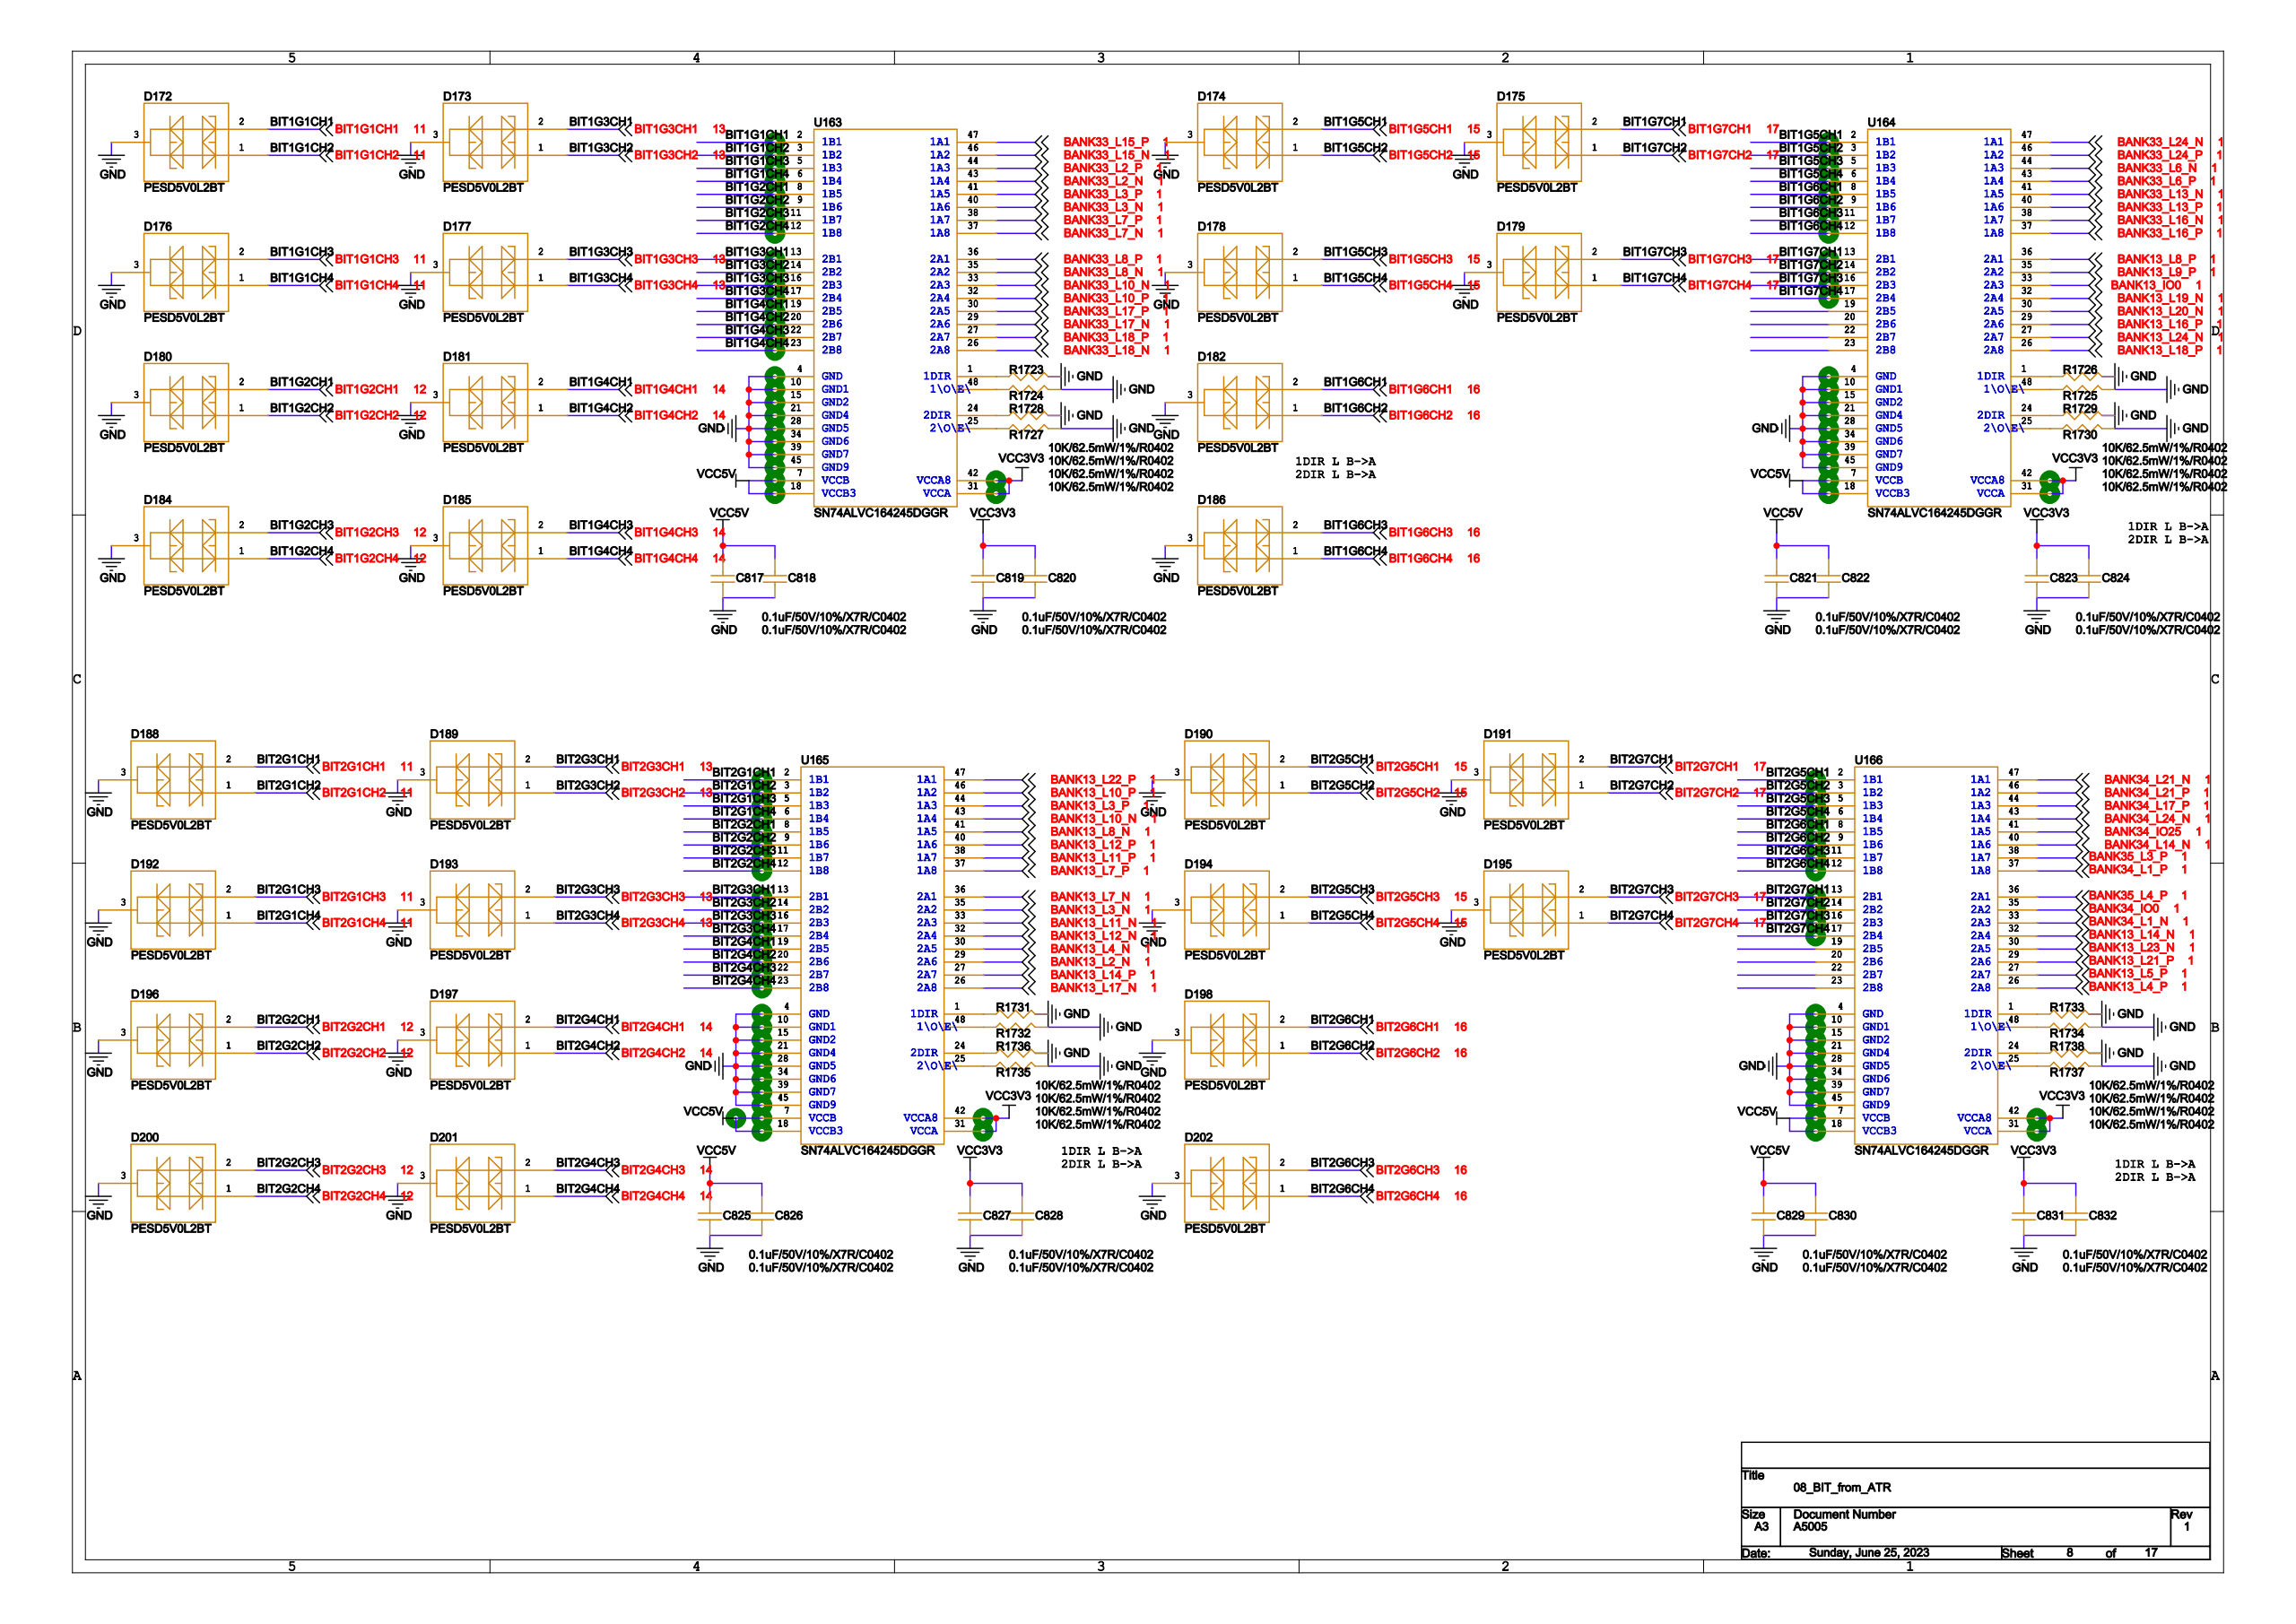Circuit board | Cadence Allegro | 1997 parts | 1536 nets | one sheet of the schematic
Parts on this sheet (reference | value | footprint):
C817 | 0.1uF/50V/10%/X7R/C0402 | 0402
C818 | 0.1uF/50V/10%/X7R/C0402 | 0402
C819 | 0.1uF/50V/10%/X7R/C0402 | 0402
C820 | 0.1uF/50V/10%/X7R/C0402 | 0402
C821 | 0.1uF/50V/10%/X7R/C0402 | 0402
C822 | 0.1uF/50V/10%/X7R/C0402 | 0402
C823 | 0.1uF/50V/10%/X7R/C0402 | 0402
C824 | 0.1uF/50V/10%/X7R/C0402 | 0402
C825 | 0.1uF/50V/10%/X7R/C0402 | 0402
C826 | 0.1uF/50V/10%/X7R/C0402 | 0402
C827 | 0.1uF/50V/10%/X7R/C0402 | 0402
C828 | 0.1uF/50V/10%/X7R/C0402 | 0402
C829 | 0.1uF/50V/10%/X7R/C0402 | 0402
C830 | 0.1uF/50V/10%/X7R/C0402 | 0402
C831 | 0.1uF/50V/10%/X7R/C0402 | 0402
C832 | 0.1uF/50V/10%/X7R/C0402 | 0402
D172 | PESD5V0L2BT | SOT23
D173 | PESD5V0L2BT | SOT23
D174 | PESD5V0L2BT | SOT23
D175 | PESD5V0L2BT | SOT23
D176 | PESD5V0L2BT | SOT23
D177 | PESD5V0L2BT | SOT23
D178 | PESD5V0L2BT | SOT23
D179 | PESD5V0L2BT | SOT23
D180 | PESD5V0L2BT | SOT23
D181 | PESD5V0L2BT | SOT23
D182 | PESD5V0L2BT | SOT23
D184 | PESD5V0L2BT | SOT23
D185 | PESD5V0L2BT | SOT23
D186 | PESD5V0L2BT | SOT23
D188 | PESD5V0L2BT | SOT23
D189 | PESD5V0L2BT | SOT23
D190 | PESD5V0L2BT | SOT23
D191 | PESD5V0L2BT | SOT23
D192 | PESD5V0L2BT | SOT23
D193 | PESD5V0L2BT | SOT23
D194 | PESD5V0L2BT | SOT23
D195 | PESD5V0L2BT | SOT23
D196 | PESD5V0L2BT | SOT23
D197 | PESD5V0L2BT | SOT23
D198 | PESD5V0L2BT | SOT23
D200 | PESD5V0L2BT | SOT23
D201 | PESD5V0L2BT | SOT23
D202 | PESD5V0L2BT | SOT23
R1723 | 10K/62.5mW/1%/R0402 | 0402
R1724 | 10K/62.5mW/1%/R0402 | 0402
R1725 | 10K/62.5mW/1%/R0402 | 0402
R1726 | 10K/62.5mW/1%/R0402 | 0402
R1727 | 10K/62.5mW/1%/R0402 | 0402
R1728 | 10K/62.5mW/1%/R0402 | 0402
R1729 | 10K/62.5mW/1%/R0402 | 0402
R1730 | 10K/62.5mW/1%/R0402 | 0402
R1731 | 10K/62.5mW/1%/R0402 | 0402
R1732 | 10K/62.5mW/1%/R0402 | 0402
R1733 | 10K/62.5mW/1%/R0402 | 0402
R1734 | 10K/62.5mW/1%/R0402 | 0402
R1735 | 10K/62.5mW/1%/R0402 | 0402
R1736 | 10K/62.5mW/1%/R0402 | 0402
R1737 | 10K/62.5mW/1%/R0402 | 0402
R1738 | 10K/62.5mW/1%/R0402 | 0402
U163 | SN74ALVC164245DGGR | TSSOP-48
U164 | SN74ALVC164245DGGR | TSSOP-48
U165 | SN74ALVC164245DGGR | TSSOP-48
U166 | SN74ALVC164245DGGR | TSSOP-48
Nets of these parts (net: part-pin ...):
3.3V: C819-2 C820-2 C823-2 C824-2 C827-2 C828-2 C831-2 C832-2 U163-31 U163-42 U164-31 U164-42 U165-31 U165-42 U166-31 U166-42
AGND: C817-1 C818-1 C819-1 C820-1 C821-1 C822-1 C823-1 C824-1 C825-1 C826-1 C827-1 C828-1 C829-1 C830-1 C831-1 C832-1 D172-3 D173-3 D174-3 D175-3 D176-3 D177-3 D178-3 D179-3 D180-3 D181-3 D182-3 D184-3 D185-3 D186-3 D188-3 D189-3 D190-3 D191-3 D192-3 D193-3 D194-3 D195-3 D196-3 D197-3 D198-3 D200-3 D201-3 D202-3 R1723-1 R1724-1 R1725-1 R1726-1 R1727-1 R1728-1 R1729-1 R1730-1 R1731-1 R1732-1 R1733-1 R1734-1 R1735-1 R1736-1 R1737-1 R1738-1 U163-4 U163-10 U163-15 U163-21 U163-28 U163-34 U163-39 U163-45 U164-4 U164-10 U164-15 U164-21 U164-28 U164-34 U164-39 U164-45 U165-4 U165-10 U165-15 U165-21 U165-28 U165-34 U165-39 U165-45 U166-4 U166-10 U166-15 U166-21 U166-28 U166-34 U166-39 U166-45
BANK33_L10_P: U163-32
BANK33_L17_P: U163-30
BANK33_L17_N: U163-29
BANK13_L4_P: U166-26
BANK33_L18_P: U163-27
BANK13_L5_P: U166-27
BANK33_L18_N: U163-26
BANK13_L21_P: U166-29
BANK13_L23_N: U166-30
BANK13_L14_N: U166-32
BANK34_L1_N: U166-33
BANK34_L21_P: U166-46
BANK34_L17_P: U166-44
BANK34_L24_N: U166-43
BANK34_IO25: U166-41
BANK34_L14_N: U166-40
BANK35_L3_P: U166-38
BANK34_L1_P: U166-37
BANK34_IO0: U166-35
BANK35_L4_P: U166-36
BANK34_L21_N: U166-47
BANK13_L22_P: U165-47
BANK13_L10_P: U165-46
BANK13_L3_P: U165-44
BANK13_L10_N: U165-43
BANK13_L8_N: U165-41
BANK13_L12_P: U165-40
BANK13_L11_P: U165-38
BANK13_L7_P: U165-37
BANK13_L7_N: U165-36
BANK13_L3_N: U165-35
BANK13_L11_N: U165-33
BANK13_L12_N: U165-32
BANK13_L4_N: U165-30
BANK13_L2_N: U165-29
BANK13_L14_P: U165-27
BANK13_L18_P: U164-26
BANK13_L17_N: U165-26
BANK13_L24_N: U164-27
BANK13_L16_P: U164-29
BANK13_L20_N: U164-30
BANK13_L19_N: U164-32
BANK13_IO0: U164-33
BANK13_L9_P: U164-35
BANK13_L8_P: U164-36
BANK33_L15_P: U163-47
BANK33_L16_P: U164-37
BANK33_L15_N: U163-46
BANK33_L16_N: U164-38
BANK33_L2_P: U163-44
BANK33_L13_P: U164-40
BANK33_L2_N: U163-43
BANK33_L13_N: U164-41
BANK33_L3_P: U163-41
BANK33_L6_P: U164-43
BANK33_L3_N: U163-40
BANK33_L6_N: U164-44
BANK33_L7_P: U163-38
BANK33_L24_P: U164-46
BANK33_L7_N: U163-37
BANK33_L24_N: U164-47
BANK33_L8_P: U163-36
BANK33_L8_N: U163-35
BANK33_L10_N: U163-33
VCC5V: C817-2 C818-2 C821-2 C822-2 C825-2 C826-2 C829-2 C830-2 U163-7 U163-18 U164-7 U164-18 U165-7 U165-18 U166-7 U166-18
BIT1G1CH1: D172-2 U163-2
BIT2G1CH1: D188-2 U165-2
BIT1G1CH2: D172-1 U163-3
BIT2G1CH2: D188-1 U165-3
BIT1G1CH4: D176-1 U163-6
BIT2G1CH4: D192-1 U165-6
BIT1G1CH3: D176-2 U163-5
BIT2G1CH3: D192-2 U165-5
BIT1G2CH2: D180-1 U163-9
BIT2G2CH2: D196-1 U165-9
BIT1G2CH4: D184-1 U163-12
BIT2G2CH4: D200-1 U165-12
BIT1G2CH3: D184-2 U163-11
BIT2G2CH3: D200-2 U165-11
BIT1G2CH1: D180-2 U163-8
BIT2G2CH1: D196-2 U165-8
BIT1G3CH2: D173-1 U163-14
BIT2G3CH2: D189-1 U165-14
BIT1G3CH4: D177-1 U163-17
BIT2G3CH4: D193-1 U165-17
BIT1G3CH3: D177-2 U163-16
BIT2G3CH3: D193-2 U165-16
BIT1G3CH1: D173-2 U163-13
BIT2G3CH1: D189-2 U165-13
BIT1G4CH2: D181-1 U163-20
BIT2G4CH2: D197-1 U165-20
BIT1G4CH4: D185-1 U163-23
BIT2G4CH4: D201-1 U165-23
BIT1G4CH3: D185-2 U163-22
BIT2G4CH3: D201-2 U165-22
BIT1G4CH1: D181-2 U163-19
BIT2G4CH1: D197-2 U165-19
BIT1G5CH2: D174-1 U164-3
BIT2G5CH2: D190-1 U166-3
BIT1G5CH4: D178-1 U164-6
BIT2G5CH4: D194-1 U166-6
BIT1G5CH3: D178-2 U164-5
BIT2G5CH3: D194-2 U166-5
BIT1G5CH1: D174-2 U164-2
BIT2G5CH1: D190-2 U166-2
BIT1G6CH2: D182-1 U164-9
BIT2G6CH2: D198-1 U166-9
BIT1G6CH4: D186-1 U164-12
BIT2G6CH4: D202-1 U166-12
BIT1G6CH3: D186-2 U164-11
BIT2G6CH3: D202-2 U166-11
BIT1G6CH1: D182-2 U164-8
BIT2G6CH1: D198-2 U166-8
BIT1G7CH2: D175-1 U164-14
BIT2G7CH2: D191-1 U166-14
BIT1G7CH4: D179-1 U164-17
BIT2G7CH4: D195-1 U166-17
BIT1G7CH3: D179-2 U164-16
BIT2G7CH3: D195-2 U166-16
BIT1G7CH1: D175-2 U164-13
BIT2G7CH1: D191-2 U166-13
N240386151: R1723-2 U163-1
N2403877347: R1724-2 U163-48
N2404532347: R1725-2 U164-48
N240451651: R1726-2 U164-1
N240386071: R1727-2 U163-25
N240385751: R1728-2 U163-24
N240451251: R1729-2 U164-24
N240451571: R1730-2 U164-25
N240482211: R1731-2 U165-1
N2404837947: R1732-2 U165-48
N240490171: R1733-2 U166-1
N2404917547: R1734-2 U166-48
N240482131: R1735-2 U165-25
N240481811: R1736-2 U165-24
N240490091: R1737-2 U166-25
N240489771: R1738-2 U166-24